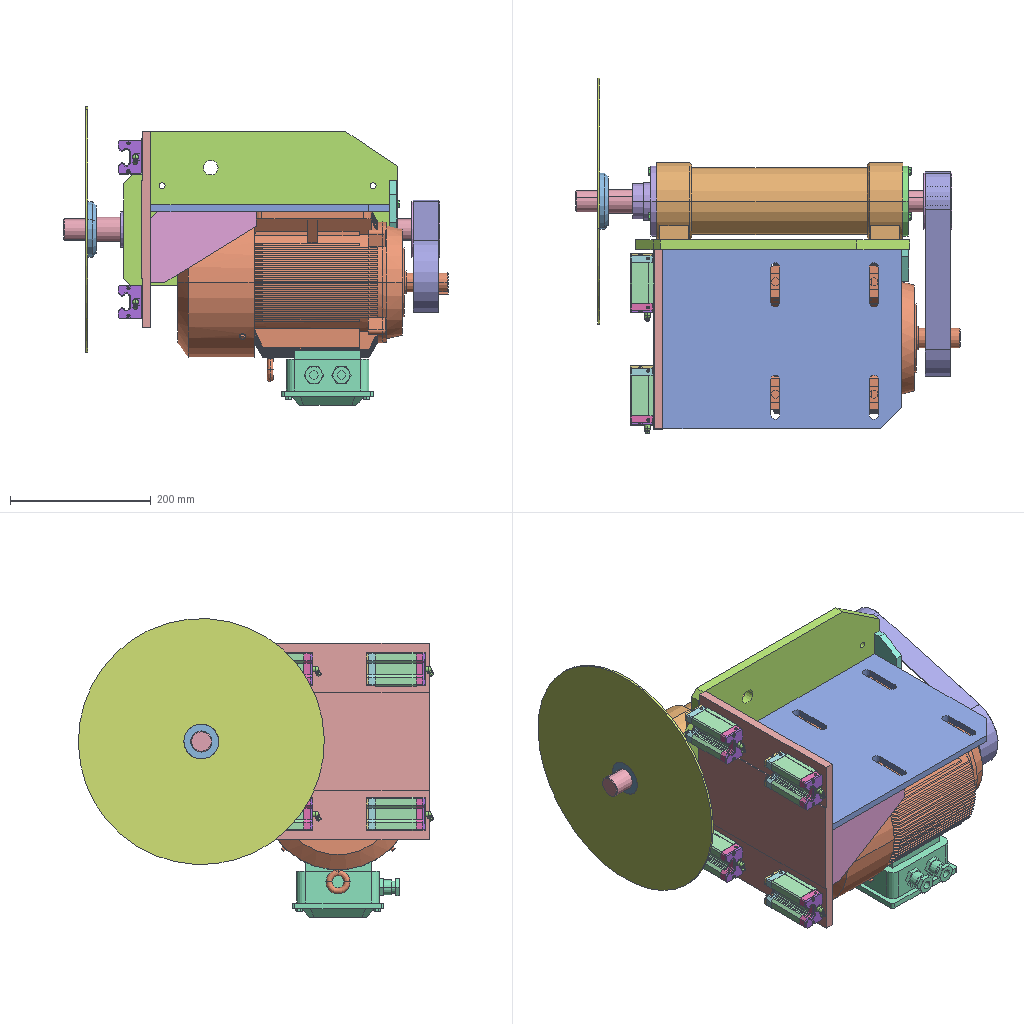Assembly | SolidWorks | 20 different items | 28 placed | box 547 x 505 x 425 mm
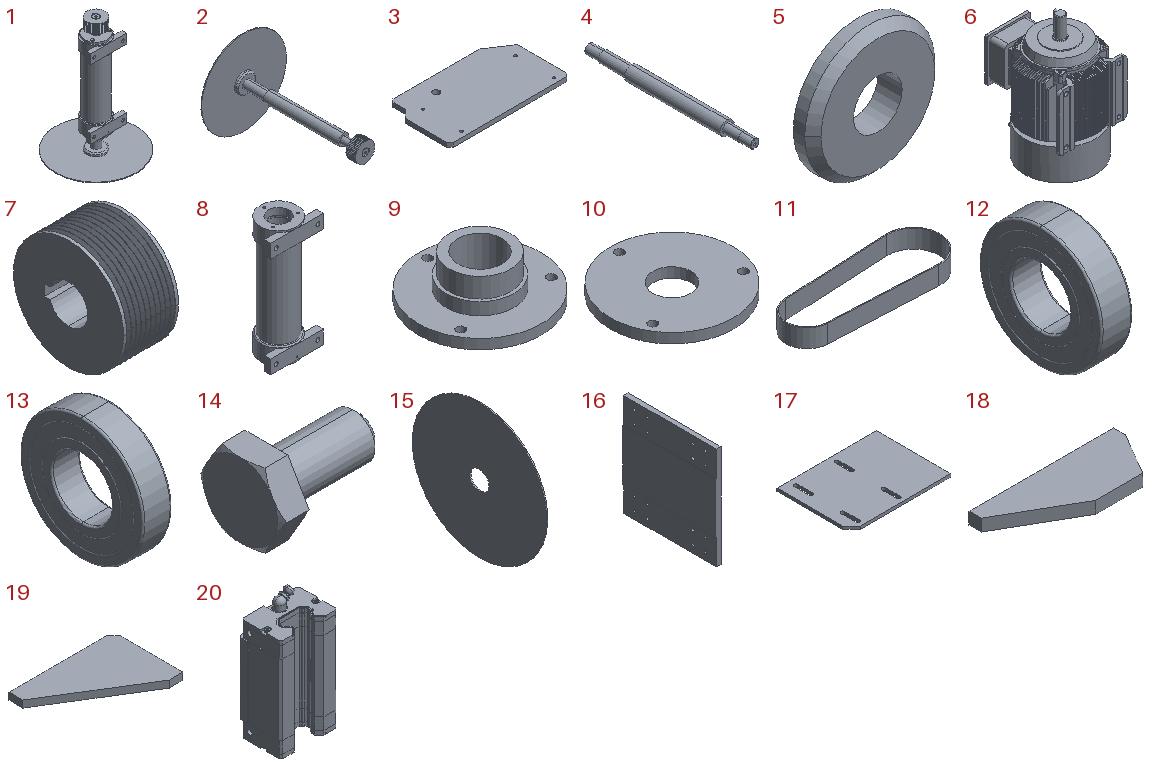Parts list (item | name | quantity | parent item | size | volume | features):
1 | (subassembly) | x1 | - | 350 x 350 x 535 mm | 3158794 mm3 | features CompositeCurve 3
2 | (subassembly) | x1 | in 1 | 350 x 535 x 350 mm | 1155640 mm3 | -
3 | - | x1 | - | 390 x 220 x 14 mm | 1142948 mm3 | features ICE 2, Chamfer 1, Extrusion 1, HoleWzd 1
4 | - | x1 | in 2 | 45 x 535 x 45 mm | 668255 mm3 | features 3DProfileFeature 1, Chamfer 1, Cut 1, HoleWzd 1, Revolution 1
5 | - | x1 | in 2 | 80 x 15 x 80 mm | 46941 mm3 | features Revolution 1
6 | - | x1 | - | 215 x 282.5 x 385 mm | 11501075 mm3 | features ICE 22, CirPattern 4, Revolution 4, Fillet 3, MoveCopyBody 3, Chamfer 2, PLine 2, DeleteBody 1, LPattern 1, SketchPattern 1
7 | - | x1 | in 2 | 39.93 x 80 x 80 mm | 157702 mm3 | features ICE 1, Revolution 1
8 | - | x1 | in 1 | 157 x 110 x 350 mm | 1792714 mm3 | features ICE 8, Chamfer 1, Extrusion 1
9 | - | x1 | in 1 | 100 x 100 x 34 mm | 82475 mm3 | features ICE 2, Extrusion 1
10 | - | x1 | in 1 | 100 x 100 x 8 mm | 55870 mm3 | features Extrusion 1
11 | - | x1 | - | 301.927 x 103.927 x 35.6 mm | 49313 mm3 | features Extrusion 1
12 | - | x1 | in 1 | 16 x 62 x 62 mm | 27684 mm3 | features Revolution 5, CirPattern 2, RefAxis 1, RevCut 1
13 | - | x1 | in 1 | 17 x 72 x 72 mm | 40403 mm3 | features Revolution 5, CirPattern 2, RefAxis 1, RevCut 1
14 | - | x6 | in 1 | 16 x 11.547 x 10 mm | 667.282 mm3 | features RevCut 3, Revolution 2, Chamfer 1, Extrusion 1
15 | - | x1 | in 2 | 3 x 350 x 350 mm | 282743 mm3 | features ICE 4, Chamfer 1, Extrusion 1, RevCut 1
16 | - | x1 | - | 14 x 255 x 280 mm | 920811 mm3 | features Extrusion 1, ICE 1
17 | - | x1 | - | 340 x 255 x 10 mm | 831191 mm3 | features Extrusion 1
18 | - | x1 | - | 120 x 45 x 10 mm | 39855 mm3 | features Extrusion 1
19 | - | x1 | - | 150 x 100 x 10 mm | 97500 mm3 | features Chamfer 1, Extrusion 1
20 | - | x4 | - | 48 x 34.4 x 96 mm | 105086 mm3 | features ICE 20, Extrusion 4, MirrorPattern 4, Chamfer 3, Fillet 3, MirrorSolid 3, Revolution 2, Dome 1, RevCut 1
Mates (type | each side: item.copy, entity, surface, feature):
In the top assembly
Coincident | 16.1 face plane Boss-Extrude1 | 3.1 face plane Boss-Extrude1 | 2 times
Coincident | 3.1 face plane Boss-Extrude1 | 18.1 face plane Boss-Extrude1
DistanceDim | 18.1 face plane Boss-Extrude1 | 3.1 face plane Boss-Extrude1
Coincident | 16.1 face plane Boss-Extrude1 | 17.1 face plane Boss-Extrude1
Coincident | 17.1 face plane Boss-Extrude1 | 3.1 face plane Boss-Extrude1
DistanceDim | 17.1 face plane Boss-Extrude1 | 16.1 face plane Boss-Extrude1
Coincident | 17.1 face plane Boss-Extrude1 | 18.1 face plane Boss-Extrude1
Coincident | 16.1 face plane Boss-Extrude1 | 19.1 face plane Boss-Extrude1
Coincident | 17.1 face plane Boss-Extrude1 | 19.1 face plane Boss-Extrude1
DistanceDim | 17.1 face plane Boss-Extrude1 | 19.1 face plane Boss-Extrude1
DistanceDim | 16.1 face plane Boss-Extrude1 | 3.1 face plane Boss-Extrude1
Coincident | 3.1 face plane Boss-Extrude1 | 8.1 face plane Boss-Extrude2
Concentric | 3.1 face cylinder M10 Tapped Hole1 | 8.1 face cylinder Boss-Extrude2 | 2 times
DistanceDim | 11.1 face plane Boss-Extrude1 | 7.1 face plane Revolve1
Coincident | 17.1 face plane Boss-Extrude1 | 6.1 face plane Boss-Extrude4
DistanceDim | 17.1 face plane Boss-Extrude1 | 6.1 face plane Boss-Extrude4
DistanceDim | 6.1 face plane Boss-Extrude4 | 17.1 face plane Boss-Extrude1
Concentric | 4.1 face cylinder Revolve1 | 11.1 face cylinder Boss-Extrude1
Coincident | 16.1 face plane Cut-Extrude3 | 20.1 face plane Boss-Extrude1
Concentric | 16.1 face cylinder Boss-Extrude1 | 20.1 face cylinder Cut-Revolve1
Concentric | 16.1 face cylinder Boss-Extrude1 | 20.1 face cylinder Mirror1
In subassembly 1
Coincident | 8.2 face plane Boss-Extrude1 | 9.1 face plane Boss-Extrude1
Concentric | 8.2 face cylinder Boss-Extrude1 | 9.1 face cylinder Boss-Extrude3
Concentric | 8.2 face cylinder Boss-Extrude1 | 10.1 face cylinder Boss-Extrude1
Coincident | 8.2 face plane Boss-Extrude1 | 10.1 face plane Boss-Extrude1
Concentric | 8.2 face cylinder Cut-Extrude6 | 10.1 face cylinder Boss-Extrude1
Concentric | 8.2 face cylinder Cut-Extrude5 | 9.1 face cylinder Boss-Extrude1
Concentric | 8.2 face cylinder Cut-Extrude3 | 12.1 face cylinder Revolve1
Coincident | 8.2 face plane Cut-Extrude1 | 12.1 face plane Revolve1
Concentric | 8.2 edge | 13.1 face cylinder Revolve1
Coincident | 8.2 face plane Cut-Extrude3 | 13.1 face plane Revolve1
Concentric | 9.1 face cylinder Boss-Extrude1 | 14.1 face cylinder Boss-Revolve1
Coincident | 9.1 face plane Boss-Extrude1 | 14.1 face plane Base-extrude
Coincident | 14.2 face plane Base-extrude | 14.3 face plane Base-extrude
Coincident | 14.1 face plane Base-extrude | 14.3 face plane Base-extrude
Concentric | 9.1 face cylinder Boss-Extrude1 | 14.2 face cylinder Boss-Revolve1
Concentric | 9.1 edge | 14.3 face cylinder Boss-Revolve1
Coincident | 14.4 face plane Base-extrude | 14.5 face plane Base-extrude
Coincident | 14.5 face plane Base-extrude | 14.6 face plane Base-extrude
Concentric | 10.1 face cylinder Boss-Extrude1 | 14.4 face cylinder Boss-Revolve1
Concentric | 10.1 edge | 14.5 face cylinder Boss-Revolve1
Concentric | 10.1 face cylinder Boss-Extrude1 | 14.6 face cylinder Boss-Revolve1
Coincident | 10.1 face plane Boss-Extrude1 | 14.4 face plane Base-extrude
Coincident | 13.1 face plane Revolve1 | 1.1 face
Concentric | 13.1 face cylinder Revolve1 | 1.1 face
Coincident | 13.1 face plane Revolve1 | 4.2 face plane Revolve1
Concentric | 13.1 face cylinder Revolve1 | 4.2 face cylinder Revolve1
In subassembly 2
Concentric | 4.3 face cylinder Revolve1 | 15.1 face cylinder Cut-Revolve1
Coincident | 5.1 face plane Revolve1 | 15.1 face plane Cut-Extrude2
Coincident | 4.3 face plane Revolve1 | 5.1 face plane Revolve1
Concentric | 4.3 face cylinder Revolve1 | 5.1 face cylinder Revolve1
Concentric | 4.3 face cylinder Revolve1 | 7.2 face cylinder Cut-Extrude1
Coincident | 4.3 face plane Revolve1 | 7.2 face plane Revolve1